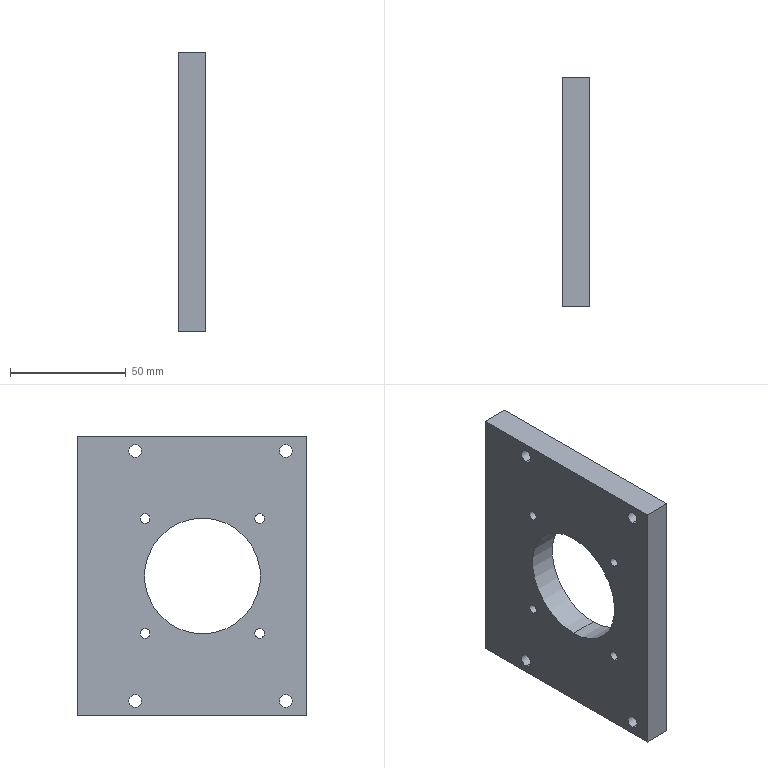Part | STEP file | 0245_201_Plate | 1 solid | 32 faces | box 12 x 99 x 120 mm | volume 116837 mm3 | cylinder 22 | plane 6 | cone 4 | commonest cylinder face diameters 4.2 x12 5.5 x8 50 x2